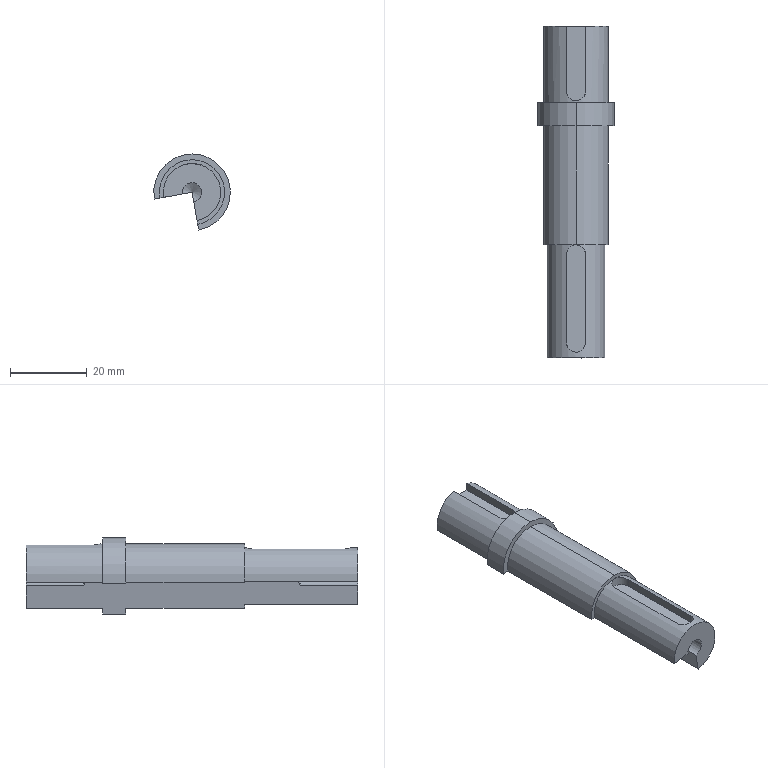Part | STEP file | Cuon T phu H01_21 | 1 solid | 28 faces | box 20 x 86.57 x 19.844 mm | volume 13014 mm3 | plane 13 | cylinder 12 | cone 3 | commonest cylinder face diameters 5 x6 17 x3 20 x2 15 x1